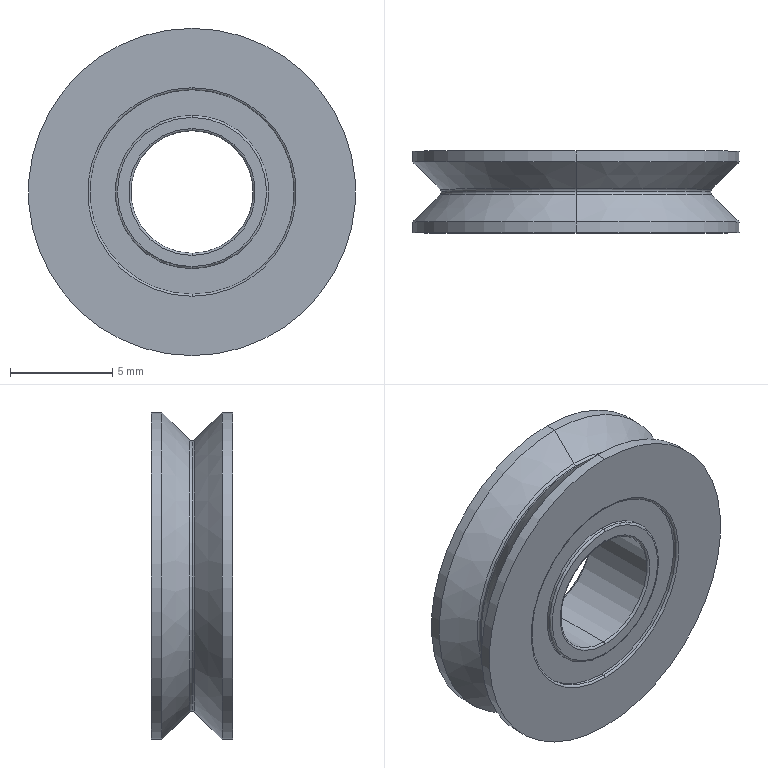Part | NX | features BREP 1 | 1 solid | 40 faces | box 16 x 4 x 16 mm | volume 572.042 mm3 | torus 16 | cylinder 14 | plane 6 | cone 4 | commonest cylinder face diameters 7.5 x4 10 x4 16 x4 6 x2
STEP:
#1=CARTESIAN_POINT('',(0.,2.,-6.613));
#2=VERTEX_POINT('',#1);
#3=CARTESIAN_POINT('',(0.,2.,6.613));
#4=VERTEX_POINT('',#3);
#5=CARTESIAN_POINT('',(0.,2.,0.));
#6=DIRECTION('',(0.,-1.,0.));
#7=DIRECTION('',(0.,0.,-1.));
#8=AXIS2_PLACEMENT_3D('',#5,#6,#7);
#9=CIRCLE('',#8,6.613);
#10=EDGE_CURVE('',#2,#4,#9,.T.);
#11=ORIENTED_EDGE('',*,*,#10,.F.);
#12=CARTESIAN_POINT('',(0.,2.141,-6.671));
#13=VERTEX_POINT('',#12);
#14=CARTESIAN_POINT('',(0.,2.,-6.813));
#15=DIRECTION('',(-1.,0.,0.));
#16=DIRECTION('',(0.,0.,1.));
#17=AXIS2_PLACEMENT_3D('',#14,#15,#16);
#18=CIRCLE('',#17,0.2);
#19=EDGE_CURVE('',#2,#13,#18,.T.);
#20=ORIENTED_EDGE('',*,*,#19,.T.);
#21=CARTESIAN_POINT('',(0.,2.141,6.671));
#22=VERTEX_POINT('',#21);
#23=CARTESIAN_POINT('',(0.,2.141,0.));
#24=DIRECTION('',(0.,1.,0.));
#25=DIRECTION('',(0.,0.,1.));
#26=AXIS2_PLACEMENT_3D('',#23,#24,#25);
#27=CIRCLE('',#26,6.671);
#28=EDGE_CURVE('',#22,#13,#27,.T.);
#29=ORIENTED_EDGE('',*,*,#28,.F.);
#30=CARTESIAN_POINT('',(0.,2.,6.813));
#31=DIRECTION('',(1.,0.,0.));
#32=DIRECTION('',(0.,0.,-1.));
#33=AXIS2_PLACEMENT_3D('',#30,#31,#32);
#34=CIRCLE('',#33,0.2);
#35=EDGE_CURVE('',#4,#22,#34,.T.);
#36=ORIENTED_EDGE('',*,*,#35,.F.);
#37=EDGE_LOOP('',(#11,#20,#29,#36));
#38=FACE_BOUND('',#37,.T.);
#39=CARTESIAN_POINT('',(0.,2.,0.));
#40=DIRECTION('',(0.,-1.,0.));
#41=DIRECTION('',(0.,0.,-1.));
#42=AXIS2_PLACEMENT_3D('',#39,#40,#41);
#43=TOROIDAL_SURFACE('',#42,6.813,0.2);
#44=ADVANCED_FACE('',(#38),#43,.F.);
#45=CARTESIAN_POINT('',(0.,3.9,-3.));
#46=VERTEX_POINT('',#45);
#47=CARTESIAN_POINT('',(0.,4.,-3.1));
#48=VERTEX_POINT('',#47);
#49=CARTESIAN_POINT('',(0.,3.9,-3.1));
#50=DIRECTION('',(1.,0.,0.));
#51=DIRECTION('',(0.,0.,-1.));
#52=AXIS2_PLACEMENT_3D('',#49,#50,#51);
#53=CIRCLE('',#52,0.1);
#54=EDGE_CURVE('',#46,#48,#53,.F.);
#55=ORIENTED_EDGE('',*,*,#54,.T.);
#56=CARTESIAN_POINT('',(0.,4.,3.1));
#57=VERTEX_POINT('',#56);
#58=CARTESIAN_POINT('',(0.,4.,0.));
#59=DIRECTION('',(0.,-1.,0.));
#60=DIRECTION('',(0.,0.,1.));
#61=AXIS2_PLACEMENT_3D('',#58,#59,#60);
#62=CIRCLE('',#61,3.1);
#63=EDGE_CURVE('',#57,#48,#62,.T.);
#64=ORIENTED_EDGE('',*,*,#63,.F.);
#65=CARTESIAN_POINT('',(0.,3.9,3.));
#66=VERTEX_POINT('',#65);
#67=CARTESIAN_POINT('',(0.,3.9,3.1));
#68=DIRECTION('',(-1.,0.,0.));
#69=DIRECTION('',(0.,0.,1.));
#70=AXIS2_PLACEMENT_3D('',#67,#68,#69);
#71=CIRCLE('',#70,0.1);
#72=EDGE_CURVE('',#66,#57,#71,.F.);
#73=ORIENTED_EDGE('',*,*,#72,.F.);
#74=CARTESIAN_POINT('',(0.,3.9,0.));
#75=DIRECTION('',(0.,1.,0.));
#76=DIRECTION('',(0.,0.,1.));
#77=AXIS2_PLACEMENT_3D('',#74,#75,#76);
#78=CIRCLE('',#77,3.);
#79=EDGE_CURVE('',#46,#66,#78,.T.);
#80=ORIENTED_EDGE('',*,*,#79,.F.);
#81=EDGE_LOOP('',(#55,#64,#73,#80));
#82=FACE_BOUND('',#81,.T.);
#83=CARTESIAN_POINT('',(0.,3.9,0.));
#84=DIRECTION('',(0.,1.,0.));
#85=DIRECTION('',(0.,0.,1.));
#86=AXIS2_PLACEMENT_3D('',#83,#84,#85);
#87=TOROIDAL_SURFACE('',#86,3.1,0.1);
#88=ADVANCED_FACE('',(#82),#87,.T.);
#89=CARTESIAN_POINT('',(0.,0.,3.1));
#90=VERTEX_POINT('',#89);
#91=CARTESIAN_POINT('',(0.,0.1,3.));
#92=VERTEX_POINT('',#91);
#93=CARTESIAN_POINT('',(0.,0.1,3.1));
#94=DIRECTION('',(1.,0.,0.));
#95=DIRECTION('',(0.,0.,-1.));
#96=AXIS2_PLACEMENT_3D('',#93,#94,#95);
#97=CIRCLE('',#96,0.1);
#98=EDGE_CURVE('',#90,#92,#97,.T.);
#99=ORIENTED_EDGE('',*,*,#98,.F.);
#100=CARTESIAN_POINT('',(0.,0.,-3.1));
#101=VERTEX_POINT('',#100);
#102=CARTESIAN_POINT('',(0.,0.,0.));
#103=DIRECTION('',(0.,1.,0.));
#104=DIRECTION('',(0.,0.,-1.));
#105=AXIS2_PLACEMENT_3D('',#102,#103,#104);
#106=CIRCLE('',#105,3.1);
#107=EDGE_CURVE('',#101,#90,#106,.T.);
#108=ORIENTED_EDGE('',*,*,#107,.F.);
#109=CARTESIAN_POINT('',(0.,0.1,-3.));
#110=VERTEX_POINT('',#109);
#111=CARTESIAN_POINT('',(0.,0.1,-3.1));
#112=DIRECTION('',(-1.,0.,0.));
#113=DIRECTION('',(0.,0.,1.));
#114=AXIS2_PLACEMENT_3D('',#111,#112,#113);
#115=CIRCLE('',#114,0.1);
#116=EDGE_CURVE('',#101,#110,#115,.T.);
#117=ORIENTED_EDGE('',*,*,#116,.T.);
#118=CARTESIAN_POINT('',(0.,0.1,0.));
#119=DIRECTION('',(0.,-1.,0.));
#120=DIRECTION('',(0.,0.,-1.));
#121=AXIS2_PLACEMENT_3D('',#118,#119,#120);
#122=CIRCLE('',#121,3.);
#123=EDGE_CURVE('',#92,#110,#122,.T.);
#124=ORIENTED_EDGE('',*,*,#123,.F.);
#125=EDGE_LOOP('',(#99,#108,#117,#124));
#126=FACE_BOUND('',#125,.T.);
#127=CARTESIAN_POINT('',(0.,0.1,0.));
#128=DIRECTION('',(0.,-1.,0.));
#129=DIRECTION('',(0.,0.,-1.));
#130=AXIS2_PLACEMENT_3D('',#127,#128,#129);
#131=TOROIDAL_SURFACE('',#130,3.1,0.1);
#132=ADVANCED_FACE('',(#126),#131,.T.);
#133=CARTESIAN_POINT('',(0.,4.,-3.65));
#134=VERTEX_POINT('',#133);
#135=CARTESIAN_POINT('',(0.,3.9,-3.75));
#136=VERTEX_POINT('',#135);
#137=CARTESIAN_POINT('',(0.,3.9,-3.65));
#138=DIRECTION('',(1.,0.,0.));
#139=DIRECTION('',(0.,0.,-1.));
#140=AXIS2_PLACEMENT_3D('',#137,#138,#139);
#141=CIRCLE('',#140,0.1);
#142=EDGE_CURVE('',#134,#136,#141,.F.);
#143=ORIENTED_EDGE('',*,*,#142,.T.);
#144=CARTESIAN_POINT('',(0.,3.9,3.75));
#145=VERTEX_POINT('',#144);
#146=CARTESIAN_POINT('',(0.,3.9,0.));
#147=DIRECTION('',(0.,-1.,0.));
#148=DIRECTION('',(0.,0.,1.));
#149=AXIS2_PLACEMENT_3D('',#146,#147,#148);
#150=CIRCLE('',#149,3.75);
#151=EDGE_CURVE('',#145,#136,#150,.T.);
#152=ORIENTED_EDGE('',*,*,#151,.F.);
#153=CARTESIAN_POINT('',(0.,4.,3.65));
#154=VERTEX_POINT('',#153);
#155=CARTESIAN_POINT('',(0.,3.9,3.65));
#156=DIRECTION('',(-1.,0.,0.));
#157=DIRECTION('',(0.,0.,1.));
#158=AXIS2_PLACEMENT_3D('',#155,#156,#157);
#159=CIRCLE('',#158,0.1);
#160=EDGE_CURVE('',#154,#145,#159,.F.);
#161=ORIENTED_EDGE('',*,*,#160,.F.);
#162=CARTESIAN_POINT('',(0.,4.,0.));
#163=DIRECTION('',(0.,1.,0.));
#164=DIRECTION('',(0.,0.,1.));
#165=AXIS2_PLACEMENT_3D('',#162,#163,#164);
#166=CIRCLE('',#165,3.65);
#167=EDGE_CURVE('',#134,#154,#166,.T.);
#168=ORIENTED_EDGE('',*,*,#167,.F.);
#169=EDGE_LOOP('',(#143,#152,#161,#168));
#170=FACE_BOUND('',#169,.T.);
#171=CARTESIAN_POINT('',(0.,3.9,0.));
#172=DIRECTION('',(0.,1.,0.));
#173=DIRECTION('',(0.,0.,1.));
#174=AXIS2_PLACEMENT_3D('',#171,#172,#173);
#175=TOROIDAL_SURFACE('',#174,3.65,0.1);
#176=ADVANCED_FACE('',(#170),#175,.T.);
#177=CARTESIAN_POINT('',(0.,3.9,-5.));
#178=VERTEX_POINT('',#177);
#179=CARTESIAN_POINT('',(0.,4.,-5.1));
#180=VERTEX_POINT('',#179);
#181=CARTESIAN_POINT('',(0.,3.9,-5.1));
#182=DIRECTION('',(1.,0.,0.));
#183=DIRECTION('',(0.,0.,-1.));
#184=AXIS2_PLACEMENT_3D('',#181,#182,#183);
#185=CIRCLE('',#184,0.1);
#186=EDGE_CURVE('',#178,#180,#185,.F.);
#187=ORIENTED_EDGE('',*,*,#186,.T.);
#188=CARTESIAN_POINT('',(0.,4.,5.1));
#189=VERTEX_POINT('',#188);
#190=CARTESIAN_POINT('',(0.,4.,0.));
#191=DIRECTION('',(0.,-1.,0.));
#192=DIRECTION('',(0.,0.,1.));
#193=AXIS2_PLACEMENT_3D('',#190,#191,#192);
#194=CIRCLE('',#193,5.1);
#195=EDGE_CURVE('',#189,#180,#194,.T.);
#196=ORIENTED_EDGE('',*,*,#195,.F.);
#197=CARTESIAN_POINT('',(0.,3.9,5.));
#198=VERTEX_POINT('',#197);
#199=CARTESIAN_POINT('',(0.,3.9,5.1));
#200=DIRECTION('',(-1.,0.,0.));
#201=DIRECTION('',(0.,0.,1.));
#202=AXIS2_PLACEMENT_3D('',#199,#200,#201);
#203=CIRCLE('',#202,0.1);
#204=EDGE_CURVE('',#198,#189,#203,.F.);
#205=ORIENTED_EDGE('',*,*,#204,.F.);
#206=CARTESIAN_POINT('',(0.,3.9,0.));
#207=DIRECTION('',(0.,1.,0.));
#208=DIRECTION('',(0.,0.,1.));
#209=AXIS2_PLACEMENT_3D('',#206,#207,#208);
#210=CIRCLE('',#209,5.);
#211=EDGE_CURVE('',#178,#198,#210,.T.);
#212=ORIENTED_EDGE('',*,*,#211,.F.);
#213=EDGE_LOOP('',(#187,#196,#205,#212));
#214=FACE_BOUND('',#213,.T.);
#215=CARTESIAN_POINT('',(0.,3.9,0.));
#216=DIRECTION('',(0.,1.,0.));
#217=DIRECTION('',(0.,0.,1.));
#218=AXIS2_PLACEMENT_3D('',#215,#216,#217);
#219=TOROIDAL_SURFACE('',#218,5.1,0.1);
#220=ADVANCED_FACE('',(#214),#219,.T.);
#221=CARTESIAN_POINT('',(0.,0.1,3.75));
#222=VERTEX_POINT('',#221);
#223=CARTESIAN_POINT('',(0.,0.,3.65));
#224=VERTEX_POINT('',#223);
#225=CARTESIAN_POINT('',(0.,0.1,3.65));
#226=DIRECTION('',(1.,0.,0.));
#227=DIRECTION('',(0.,0.,-1.));
#228=AXIS2_PLACEMENT_3D('',#225,#226,#227);
#229=CIRCLE('',#228,0.1);
#230=EDGE_CURVE('',#222,#224,#229,.T.);
#231=ORIENTED_EDGE('',*,*,#230,.F.);
#232=CARTESIAN_POINT('',(0.,0.1,-3.75));
#233=VERTEX_POINT('',#232);
#234=CARTESIAN_POINT('',(0.,0.1,0.));
#235=DIRECTION('',(0.,1.,0.));
#236=DIRECTION('',(0.,0.,-1.));
#237=AXIS2_PLACEMENT_3D('',#234,#235,#236);
#238=CIRCLE('',#237,3.75);
#239=EDGE_CURVE('',#233,#222,#238,.T.);
#240=ORIENTED_EDGE('',*,*,#239,.F.);
#241=CARTESIAN_POINT('',(0.,0.,-3.65));
#242=VERTEX_POINT('',#241);
#243=CARTESIAN_POINT('',(0.,0.1,-3.65));
#244=DIRECTION('',(-1.,0.,0.));
#245=DIRECTION('',(0.,0.,1.));
#246=AXIS2_PLACEMENT_3D('',#243,#244,#245);
#247=CIRCLE('',#246,0.1);
#248=EDGE_CURVE('',#233,#242,#247,.T.);
#249=ORIENTED_EDGE('',*,*,#248,.T.);
#250=CARTESIAN_POINT('',(0.,0.,0.));
#251=DIRECTION('',(0.,-1.,0.));
#252=DIRECTION('',(0.,0.,-1.));
#253=AXIS2_PLACEMENT_3D('',#250,#251,#252);
#254=CIRCLE('',#253,3.65);
#255=EDGE_CURVE('',#224,#242,#254,.T.);
#256=ORIENTED_EDGE('',*,*,#255,.F.);
#257=EDGE_LOOP('',(#231,#240,#249,#256));
#258=FACE_BOUND('',#257,.T.);
#259=CARTESIAN_POINT('',(0.,0.1,0.));
#260=DIRECTION('',(0.,-1.,0.));
#261=DIRECTION('',(0.,0.,-1.));
#262=AXIS2_PLACEMENT_3D('',#259,#260,#261);
#263=TOROIDAL_SURFACE('',#262,3.65,0.1);
#264=ADVANCED_FACE('',(#258),#263,.T.);
#265=CARTESIAN_POINT('',(0.,0.,5.1));
#266=VERTEX_POINT('',#265);
#267=CARTESIAN_POINT('',(0.,0.1,5.));
#268=VERTEX_POINT('',#267);
#269=CARTESIAN_POINT('',(0.,0.1,5.1));
#270=DIRECTION('',(1.,0.,0.));
#271=DIRECTION('',(0.,0.,-1.));
#272=AXIS2_PLACEMENT_3D('',#269,#270,#271);
#273=CIRCLE('',#272,0.1);
#274=EDGE_CURVE('',#266,#268,#273,.T.);
#275=ORIENTED_EDGE('',*,*,#274,.F.);
#276=CARTESIAN_POINT('',(0.,0.,-5.1));
#277=VERTEX_POINT('',#276);
#278=CARTESIAN_POINT('',(0.,0.,0.));
#279=DIRECTION('',(0.,1.,0.));
#280=DIRECTION('',(0.,0.,-1.));
#281=AXIS2_PLACEMENT_3D('',#278,#279,#280);
#282=CIRCLE('',#281,5.1);
#283=EDGE_CURVE('',#277,#266,#282,.T.);
#284=ORIENTED_EDGE('',*,*,#283,.F.);
#285=CARTESIAN_POINT('',(0.,0.1,-5.));
#286=VERTEX_POINT('',#285);
#287=CARTESIAN_POINT('',(0.,0.1,-5.1));
#288=DIRECTION('',(-1.,0.,0.));
#289=DIRECTION('',(0.,0.,1.));
#290=AXIS2_PLACEMENT_3D('',#287,#288,#289);
#291=CIRCLE('',#290,0.1);
#292=EDGE_CURVE('',#277,#286,#291,.T.);
#293=ORIENTED_EDGE('',*,*,#292,.T.);
#294=CARTESIAN_POINT('',(0.,0.1,0.));
#295=DIRECTION('',(0.,-1.,0.));
#296=DIRECTION('',(0.,0.,-1.));
#297=AXIS2_PLACEMENT_3D('',#294,#295,#296);
#298=CIRCLE('',#297,5.);
#299=EDGE_CURVE('',#268,#286,#298,.T.);
#300=ORIENTED_EDGE('',*,*,#299,.F.);
#301=EDGE_LOOP('',(#275,#284,#293,#300));
#302=FACE_BOUND('',#301,.T.);
#303=CARTESIAN_POINT('',(0.,0.1,0.));
#304=DIRECTION('',(0.,-1.,0.));
#305=DIRECTION('',(0.,0.,-1.));
#306=AXIS2_PLACEMENT_3D('',#303,#304,#305);
#307=TOROIDAL_SURFACE('',#306,5.1,0.1);
#308=ADVANCED_FACE('',(#302),#307,.T.);
#309=CARTESIAN_POINT('',(0.,3.75,-3.75));
#310=VERTEX_POINT('',#309);
#311=CARTESIAN_POINT('',(0.,3.75,-3.75));
#312=DIRECTION('',(0.,1.,0.));
#313=VECTOR('',#312,1000.);
#314=LINE('',#311,#313);
#315=EDGE_CURVE('',#136,#310,#314,.F.);
#316=ORIENTED_EDGE('',*,*,#315,.T.);
#317=CARTESIAN_POINT('',(0.,3.75,3.75));
#318=VERTEX_POINT('',#317);
#319=CARTESIAN_POINT('',(0.,3.75,0.));
#320=DIRECTION('',(0.,1.,0.));
#321=DIRECTION('',(0.,0.,1.));
#322=AXIS2_PLACEMENT_3D('',#319,#320,#321);
#323=CIRCLE('',#322,3.75);
#324=EDGE_CURVE('',#310,#318,#323,.T.);
#325=ORIENTED_EDGE('',*,*,#324,.T.);
#326=CARTESIAN_POINT('',(0.,3.75,3.75));
#327=DIRECTION('',(0.,1.,0.));
#328=VECTOR('',#327,1000.);
#329=LINE('',#326,#328);
#330=EDGE_CURVE('',#145,#318,#329,.F.);
#331=ORIENTED_EDGE('',*,*,#330,.F.);
#332=ORIENTED_EDGE('',*,*,#151,.T.);
#333=EDGE_LOOP('',(#316,#325,#331,#332));
#334=FACE_BOUND('',#333,.T.);
#335=CARTESIAN_POINT('',(0.,3.75,0.));
#336=DIRECTION('',(0.,1.,0.));
#337=DIRECTION('',(0.,0.,1.));
#338=AXIS2_PLACEMENT_3D('',#335,#336,#337);
#339=CYLINDRICAL_SURFACE('',#338,3.75);
#340=ADVANCED_FACE('',(#334),#339,.T.);
#341=CARTESIAN_POINT('',(0.,3.75,5.));
#342=VERTEX_POINT('',#341);
#343=CARTESIAN_POINT('',(0.,3.75,-5.));
#344=VERTEX_POINT('',#343);
#345=CARTESIAN_POINT('',(0.,3.75,0.));
#346=DIRECTION('',(0.,1.,0.));
#347=DIRECTION('',(0.,0.,1.));
#348=AXIS2_PLACEMENT_3D('',#345,#346,#347);
#349=CIRCLE('',#348,5.);
#350=EDGE_CURVE('',#342,#344,#349,.T.);
#351=ORIENTED_EDGE('',*,*,#350,.T.);
#352=CARTESIAN_POINT('',(0.,3.75,0.));
#353=DIRECTION('',(0.,1.,0.));
#354=DIRECTION('',(0.,0.,1.));
#355=AXIS2_PLACEMENT_3D('',#352,#353,#354);
#356=CIRCLE('',#355,5.);
#357=EDGE_CURVE('',#344,#342,#356,.T.);
#358=ORIENTED_EDGE('',*,*,#357,.T.);
#359=EDGE_LOOP('',(#351,#358));
#360=FACE_BOUND('',#359,.T.);
#361=CARTESIAN_POINT('',(0.,3.75,0.));
#362=DIRECTION('',(0.,1.,0.));
#363=DIRECTION('',(0.,0.,1.));
#364=AXIS2_PLACEMENT_3D('',#361,#362,#363);
#365=CIRCLE('',#364,3.75);
#366=EDGE_CURVE('',#318,#310,#365,.T.);
#367=ORIENTED_EDGE('',*,*,#366,.F.);
#368=ORIENTED_EDGE('',*,*,#324,.F.);
#369=EDGE_LOOP('',(#367,#368));
#370=FACE_BOUND('',#369,.T.);
#371=CARTESIAN_POINT('',(0.,3.75,0.));
#372=DIRECTION('',(0.,1.,0.));
#373=DIRECTION('',(0.,0.,1.));
#374=AXIS2_PLACEMENT_3D('',#371,#372,#373);
#375=PLANE('',#374);
#376=ADVANCED_FACE('',(#360,#370),#375,.T.);
#377=CARTESIAN_POINT('',(0.,3.75,-5.));
#378=DIRECTION('',(0.,1.,0.));
#379=VECTOR('',#378,1000.);
#380=LINE('',#377,#379);
#381=EDGE_CURVE('',#178,#344,#380,.F.);
#382=ORIENTED_EDGE('',*,*,#381,.T.);
#383=ORIENTED_EDGE('',*,*,#350,.F.);
#384=CARTESIAN_POINT('',(0.,3.75,5.));
#385=DIRECTION('',(0.,1.,0.));
#386=VECTOR('',#385,1000.);
#387=LINE('',#384,#386);
#388=EDGE_CURVE('',#198,#342,#387,.F.);
#389=ORIENTED_EDGE('',*,*,#388,.F.);
#390=CARTESIAN_POINT('',(0.,3.9,0.));
#391=DIRECTION('',(0.,1.,0.));
#392=DIRECTION('',(0.,0.,1.));
#393=AXIS2_PLACEMENT_3D('',#390,#391,#392);
#394=CIRCLE('',#393,5.);
#395=EDGE_CURVE('',#198,#178,#394,.T.);
#396=ORIENTED_EDGE('',*,*,#395,.T.);
#397=EDGE_LOOP('',(#382,#383,#389,#396));
#398=FACE_BOUND('',#397,.T.);
#399=CARTESIAN_POINT('',(0.,3.75,0.));
#400=DIRECTION('',(0.,1.,0.));
#401=DIRECTION('',(0.,0.,1.));
#402=AXIS2_PLACEMENT_3D('',#399,#400,#401);
#403=CYLINDRICAL_SURFACE('',#402,5.);
#404=ADVANCED_FACE('',(#398),#403,.F.);
#405=CARTESIAN_POINT('',(0.,0.25,3.75));
#406=VERTEX_POINT('',#405);
#407=CARTESIAN_POINT('',(0.,0.25,3.75));
#408=DIRECTION('',(0.,-1.,0.));
#409=VECTOR('',#408,1000.);
#410=LINE('',#407,#409);
#411=EDGE_CURVE('',#406,#222,#410,.T.);
#412=ORIENTED_EDGE('',*,*,#411,.F.);
#413=CARTESIAN_POINT('',(0.,0.25,-3.75));
#414=VERTEX_POINT('',#413);
#415=CARTESIAN_POINT('',(0.,0.25,0.));
#416=DIRECTION('',(0.,-1.,0.));
#417=DIRECTION('',(0.,0.,-1.));
#418=AXIS2_PLACEMENT_3D('',#415,#416,#417);
#419=CIRCLE('',#418,3.75);
#420=EDGE_CURVE('',#406,#414,#419,.T.);
#421=ORIENTED_EDGE('',*,*,#420,.T.);
#422=CARTESIAN_POINT('',(0.,0.25,-3.75));
#423=DIRECTION('',(0.,-1.,0.));
#424=VECTOR('',#423,1000.);
#425=LINE('',#422,#424);
#426=EDGE_CURVE('',#414,#233,#425,.T.);
#427=ORIENTED_EDGE('',*,*,#426,.T.);
#428=ORIENTED_EDGE('',*,*,#239,.T.);
#429=EDGE_LOOP('',(#412,#421,#427,#428));
#430=FACE_BOUND('',#429,.T.);
#431=CARTESIAN_POINT('',(0.,0.25,0.));
#432=DIRECTION('',(0.,-1.,0.));
#433=DIRECTION('',(0.,0.,-1.));
#434=AXIS2_PLACEMENT_3D('',#431,#432,#433);
#435=CYLINDRICAL_SURFACE('',#434,3.75);
#436=ADVANCED_FACE('',(#430),#435,.T.);
#437=CARTESIAN_POINT('',(0.,0.25,-5.));
#438=VERTEX_POINT('',#437);
#439=CARTESIAN_POINT('',(0.,0.25,5.));
#440=VERTEX_POINT('',#439);
#441=CARTESIAN_POINT('',(0.,0.25,0.));
#442=DIRECTION('',(0.,-1.,0.));
#443=DIRECTION('',(0.,0.,-1.));
#444=AXIS2_PLACEMENT_3D('',#441,#442,#443);
#445=CIRCLE('',#444,5.);
#446=EDGE_CURVE('',#438,#440,#445,.T.);
#447=ORIENTED_EDGE('',*,*,#446,.T.);
#448=CARTESIAN_POINT('',(0.,0.25,0.));
#449=DIRECTION('',(0.,-1.,0.));
#450=DIRECTION('',(0.,0.,-1.));
#451=AXIS2_PLACEMENT_3D('',#448,#449,#450);
#452=CIRCLE('',#451,5.);
#453=EDGE_CURVE('',#440,#438,#452,.T.);
#454=ORIENTED_EDGE('',*,*,#453,.T.);
#455=EDGE_LOOP('',(#447,#454));
#456=FACE_BOUND('',#455,.T.);
#457=CARTESIAN_POINT('',(0.,0.25,0.));
#458=DIRECTION('',(0.,-1.,0.));
#459=DIRECTION('',(0.,0.,-1.));
#460=AXIS2_PLACEMENT_3D('',#457,#458,#459);
#461=CIRCLE('',#460,3.75);
#462=EDGE_CURVE('',#414,#406,#461,.T.);
#463=ORIENTED_EDGE('',*,*,#462,.F.);
#464=ORIENTED_EDGE('',*,*,#420,.F.);
#465=EDGE_LOOP('',(#463,#464));
#466=FACE_BOUND('',#465,.T.);
#467=CARTESIAN_POINT('',(0.,0.25,0.));
#468=DIRECTION('',(0.,-1.,0.));
#469=DIRECTION('',(0.,0.,-1.));
#470=AXIS2_PLACEMENT_3D('',#467,#468,#469);
#471=PLANE('',#470);
#472=ADVANCED_FACE('',(#456,#466),#471,.T.);
#473=CARTESIAN_POINT('',(0.,0.25,5.));
#474=DIRECTION('',(0.,-1.,0.));
#475=VECTOR('',#474,1000.);
#476=LINE('',#473,#475);
#477=EDGE_CURVE('',#440,#268,#476,.T.);
#478=ORIENTED_EDGE('',*,*,#477,.F.);
#479=ORIENTED_EDGE('',*,*,#446,.F.);
#480=CARTESIAN_POINT('',(0.,0.25,-5.));
#481=DIRECTION('',(0.,-1.,0.));
#482=VECTOR('',#481,1000.);
#483=LINE('',#480,#482);
#484=EDGE_CURVE('',#438,#286,#483,.T.);
#485=ORIENTED_EDGE('',*,*,#484,.T.);
#486=CARTESIAN_POINT('',(0.,0.1,0.));
#487=DIRECTION('',(0.,-1.,0.));
#488=DIRECTION('',(0.,0.,-1.));
#489=AXIS2_PLACEMENT_3D('',#486,#487,#488);
#490=CIRCLE('',#489,5.);
#491=EDGE_CURVE('',#286,#268,#490,.T.);
#492=ORIENTED_EDGE('',*,*,#491,.T.);
#493=EDGE_LOOP('',(#478,#479,#485,#492));
#494=FACE_BOUND('',#493,.T.);
#495=CARTESIAN_POINT('',(0.,0.25,0.));
#496=DIRECTION('',(0.,-1.,0.));
#497=DIRECTION('',(0.,0.,-1.));
#498=AXIS2_PLACEMENT_3D('',#495,#496,#497);
#499=CYLINDRICAL_SURFACE('',#498,5.);
#500=ADVANCED_FACE('',(#494),#499,.F.);
#501=CARTESIAN_POINT('',(0.,0.53,8.));
#502=VERTEX_POINT('',#501);
#503=CARTESIAN_POINT('',(0.,0.,8.));
#504=VERTEX_POINT('',#503);
#505=CARTESIAN_POINT('',(0.,0.,8.));
#506=DIRECTION('',(0.,-1.,0.));
#507=VECTOR('',#506,1000.);
#508=LINE('',#505,#507);
#509=EDGE_CURVE('',#502,#504,#508,.T.);
#510=ORIENTED_EDGE('',*,*,#509,.F.);
#511=CARTESIAN_POINT('',(0.,0.53,-8.));
#512=VERTEX_POINT('',#511);
#513=CARTESIAN_POINT('',(0.,0.53,0.));
#514=DIRECTION('',(0.,-1.,0.));
#515=DIRECTION('',(0.,0.,-1.));
#516=AXIS2_PLACEMENT_3D('',#513,#514,#515);
#517=CIRCLE('',#516,8.);
#518=EDGE_CURVE('',#502,#512,#517,.T.);
#519=ORIENTED_EDGE('',*,*,#518,.T.);
#520=CARTESIAN_POINT('',(0.,0.,-8.));
#521=VERTEX_POINT('',#520);
#522=CARTESIAN_POINT('',(0.,0.,-8.));
#523=DIRECTION('',(0.,-1.,0.));
#524=VECTOR('',#523,1000.);
#525=LINE('',#522,#524);
#526=EDGE_CURVE('',#512,#521,#525,.T.);
#527=ORIENTED_EDGE('',*,*,#526,.T.);
#528=CARTESIAN_POINT('',(0.,0.,0.));
#529=DIRECTION('',(0.,-1.,0.));
#530=DIRECTION('',(0.,0.,-1.));
#531=AXIS2_PLACEMENT_3D('',#528,#529,#530);
#532=CIRCLE('',#531,8.);
#533=EDGE_CURVE('',#504,#521,#532,.T.);
#534=ORIENTED_EDGE('',*,*,#533,.F.);
#535=EDGE_LOOP('',(#510,#519,#527,#534));
#536=FACE_BOUND('',#535,.T.);
#537=CARTESIAN_POINT('',(0.,0.,0.));
#538=DIRECTION('',(0.,-1.,0.));
#539=DIRECTION('',(0.,0.,-1.));
#540=AXIS2_PLACEMENT_3D('',#537,#538,#539);
#541=CYLINDRICAL_SURFACE('',#540,8.);
#542=ADVANCED_FACE('',(#536),#541,.T.);
#543=CARTESIAN_POINT('',(0.,1.859,6.671));
#544=VERTEX_POINT('',#543);
#545=CARTESIAN_POINT('',(0.,0.53,8.));
#546=DIRECTION('',(0.,-0.7071,0.7071));
#547=VECTOR('',#546,1000.);
#548=LINE('',#545,#547);
#549=EDGE_CURVE('',#544,#502,#548,.T.);
#550=ORIENTED_EDGE('',*,*,#549,.F.);
#551=CARTESIAN_POINT('',(0.,1.859,-6.671));
#552=VERTEX_POINT('',#551);
#553=CARTESIAN_POINT('',(0.,1.859,0.));
#554=DIRECTION('',(0.,-1.,0.));
#555=DIRECTION('',(0.,0.,-1.));
#556=AXIS2_PLACEMENT_3D('',#553,#554,#555);
#557=CIRCLE('',#556,6.671);
#558=EDGE_CURVE('',#544,#552,#557,.T.);
#559=ORIENTED_EDGE('',*,*,#558,.T.);
#560=CARTESIAN_POINT('',(0.,0.53,-8.));
#561=DIRECTION('',(0.,-0.7071,-0.7071));
#562=VECTOR('',#561,1000.);
#563=LINE('',#560,#562);
#564=EDGE_CURVE('',#552,#512,#563,.T.);
#565=ORIENTED_EDGE('',*,*,#564,.T.);
#566=ORIENTED_EDGE('',*,*,#518,.F.);
#567=EDGE_LOOP('',(#550,#559,#565,#566));
#568=FACE_BOUND('',#567,.T.);
#569=CARTESIAN_POINT('',(0.,0.53,0.));
#570=DIRECTION('',(0.,-1.,0.));
#571=DIRECTION('',(0.,0.,-1.));
#572=AXIS2_PLACEMENT_3D('',#569,#570,#571);
#573=CONICAL_SURFACE('',#572,8.,0.7854);
#574=ADVANCED_FACE('',(#568),#573,.T.);
#575=CARTESIAN_POINT('',(0.,3.47,-8.));
#576=VERTEX_POINT('',#575);
#577=CARTESIAN_POINT('',(0.,2.,-6.53));
#578=DIRECTION('',(0.,0.7071,-0.7071));
#579=VECTOR('',#578,1000.);
#580=LINE('',#577,#579);
#581=EDGE_CURVE('',#576,#13,#580,.F.);
#582=ORIENTED_EDGE('',*,*,#581,.T.);
#583=CARTESIAN_POINT('',(0.,2.141,0.));
#584=DIRECTION('',(0.,1.,0.));
#585=DIRECTION('',(0.,0.,1.));
#586=AXIS2_PLACEMENT_3D('',#583,#584,#585);
#587=CIRCLE('',#586,6.671);
#588=EDGE_CURVE('',#13,#22,#587,.T.);
#589=ORIENTED_EDGE('',*,*,#588,.T.);
#590=CARTESIAN_POINT('',(0.,3.47,8.));
#591=VERTEX_POINT('',#590);
#592=CARTESIAN_POINT('',(0.,2.,6.53));
#593=DIRECTION('',(0.,0.7071,0.7071));
#594=VECTOR('',#593,1000.);
#595=LINE('',#592,#594);
#596=EDGE_CURVE('',#591,#22,#595,.F.);
#597=ORIENTED_EDGE('',*,*,#596,.F.);
#598=CARTESIAN_POINT('',(0.,3.47,0.));
#599=DIRECTION('',(0.,-1.,0.));
#600=DIRECTION('',(0.,0.,-1.));
#601=AXIS2_PLACEMENT_3D('',#598,#599,#600);
#602=CIRCLE('',#601,8.);
#603=EDGE_CURVE('',#591,#576,#602,.T.);
#604=ORIENTED_EDGE('',*,*,#603,.T.);
#605=EDGE_LOOP('',(#582,#589,#597,#604));
#606=FACE_BOUND('',#605,.T.);
#607=CARTESIAN_POINT('',(0.,2.,0.));
#608=DIRECTION('',(0.,1.,0.));
#609=DIRECTION('',(0.,0.,1.));
#610=AXIS2_PLACEMENT_3D('',#607,#608,#609);
#611=CONICAL_SURFACE('',#610,6.53,0.7854);
#612=ADVANCED_FACE('',(#606),#611,.T.);
#613=CARTESIAN_POINT('',(0.,4.,8.));
#614=VERTEX_POINT('',#613);
#615=CARTESIAN_POINT('',(0.,0.,8.));
#616=DIRECTION('',(0.,-1.,0.));
#617=VECTOR('',#616,1000.);
#618=LINE('',#615,#617);
#619=EDGE_CURVE('',#614,#591,#618,.T.);
#620=ORIENTED_EDGE('',*,*,#619,.F.);
#621=CARTESIAN_POINT('',(0.,4.,-8.));
#622=VERTEX_POINT('',#621);
#623=CARTESIAN_POINT('',(0.,4.,0.));
#624=DIRECTION('',(0.,-1.,0.));
#625=DIRECTION('',(0.,0.,-1.));
#626=AXIS2_PLACEMENT_3D('',#623,#624,#625);
#627=CIRCLE('',#626,8.);
#628=EDGE_CURVE('',#614,#622,#627,.T.);
#629=ORIENTED_EDGE('',*,*,#628,.T.);
#630=CARTESIAN_POINT('',(0.,0.,-8.));
#631=DIRECTION('',(0.,-1.,0.));
#632=VECTOR('',#631,1000.);
#633=LINE('',#630,#632);
#634=EDGE_CURVE('',#622,#576,#633,.T.);
#635=ORIENTED_EDGE('',*,*,#634,.T.);
#636=ORIENTED_EDGE('',*,*,#603,.F.);
#637=EDGE_LOOP('',(#620,#629,#635,#636));
#638=FACE_BOUND('',#637,.T.);
#639=CARTESIAN_POINT('',(0.,0.,0.));
#640=DIRECTION('',(0.,-1.,0.));
#641=DIRECTION('',(0.,0.,-1.));
#642=AXIS2_PLACEMENT_3D('',#639,#640,#641);
#643=CYLINDRICAL_SURFACE('',#642,8.);
#644=ADVANCED_FACE('',(#638),#643,.T.);
#645=CARTESIAN_POINT('',(0.,4.,0.));
#646=DIRECTION('',(0.,-1.,0.));
#647=DIRECTION('',(0.,0.,-1.));
#648=AXIS2_PLACEMENT_3D('',#645,#646,#647);
#649=CIRCLE('',#648,8.);
#650=EDGE_CURVE('',#622,#614,#649,.T.);
#651=ORIENTED_EDGE('',*,*,#650,.F.);
#652=ORIENTED_EDGE('',*,*,#628,.F.);
#653=EDGE_LOOP('',(#651,#652));
#654=FACE_BOUND('',#653,.T.);
#655=ORIENTED_EDGE('',*,*,#195,.T.);
#656=CARTESIAN_POINT('',(0.,4.,0.));
#657=DIRECTION('',(0.,-1.,0.));
#658=DIRECTION('',(0.,0.,1.));
#659=AXIS2_PLACEMENT_3D('',#656,#657,#658);
#660=CIRCLE('',#659,5.1);
#661=EDGE_CURVE('',#180,#189,#660,.T.);
#662=ORIENTED_EDGE('',*,*,#661,.T.);
#663=EDGE_LOOP('',(#655,#662));
#664=FACE_BOUND('',#663,.T.);
#665=CARTESIAN_POINT('',(3.,4.,0.));
#666=DIRECTION('',(0.,1.,0.));
#667=DIRECTION('',(0.,0.,1.));
#668=AXIS2_PLACEMENT_3D('',#665,#666,#667);
#669=PLANE('',#668);
#670=ADVANCED_FACE('',(#654,#664),#669,.T.);
#671=CARTESIAN_POINT('',(0.,0.,3.));
#672=DIRECTION('',(0.,-1.,0.));
#673=VECTOR('',#672,1000.);
#674=LINE('',#671,#673);
#675=EDGE_CURVE('',#66,#92,#674,.T.);
#676=ORIENTED_EDGE('',*,*,#675,.F.);
#677=CARTESIAN_POINT('',(0.,3.9,0.));
#678=DIRECTION('',(0.,1.,0.));
#679=DIRECTION('',(0.,0.,1.));
#680=AXIS2_PLACEMENT_3D('',#677,#678,#679);
#681=CIRCLE('',#680,3.);
#682=EDGE_CURVE('',#66,#46,#681,.T.);
#683=ORIENTED_EDGE('',*,*,#682,.T.);
#684=CARTESIAN_POINT('',(0.,0.,-3.));
#685=DIRECTION('',(0.,-1.,0.));
#686=VECTOR('',#685,1000.);
#687=LINE('',#684,#686);
#688=EDGE_CURVE('',#46,#110,#687,.T.);
#689=ORIENTED_EDGE('',*,*,#688,.T.);
#690=CARTESIAN_POINT('',(0.,0.1,0.));
#691=DIRECTION('',(0.,-1.,0.));
#692=DIRECTION('',(0.,0.,-1.));
#693=AXIS2_PLACEMENT_3D('',#690,#691,#692);
#694=CIRCLE('',#693,3.);
#695=EDGE_CURVE('',#110,#92,#694,.T.);
#696=ORIENTED_EDGE('',*,*,#695,.T.);
#697=EDGE_LOOP('',(#676,#683,#689,#696));
#698=FACE_BOUND('',#697,.T.);
#699=CARTESIAN_POINT('',(0.,0.,0.));
#700=DIRECTION('',(0.,-1.,0.));
#701=DIRECTION('',(0.,0.,-1.));
#702=AXIS2_PLACEMENT_3D('',#699,#700,#701);
#703=CYLINDRICAL_SURFACE('',#702,3.);
#704=ADVANCED_FACE('',(#698),#703,.F.);
#705=CARTESIAN_POINT('',(0.,0.,0.));
#706=DIRECTION('',(0.,-1.,0.));
#707=DIRECTION('',(0.,0.,-1.));
#708=AXIS2_PLACEMENT_3D('',#705,#706,#707);
#709=CIRCLE('',#708,8.);
#710=EDGE_CURVE('',#521,#504,#709,.T.);
#711=ORIENTED_EDGE('',*,*,#710,.T.);
#712=ORIENTED_EDGE('',*,*,#533,.T.);
#713=EDGE_LOOP('',(#711,#712));
#714=FACE_BOUND('',#713,.T.);
#715=ORIENTED_EDGE('',*,*,#283,.T.);
#716=CARTESIAN_POINT('',(0.,0.,0.));
#717=DIRECTION('',(0.,1.,0.));
#718=DIRECTION('',(0.,0.,-1.));
#719=AXIS2_PLACEMENT_3D('',#716,#717,#718);
#720=CIRCLE('',#719,5.1);
#721=EDGE_CURVE('',#266,#277,#720,.T.);
#722=ORIENTED_EDGE('',*,*,#721,.T.);
#723=EDGE_LOOP('',(#715,#722));
#724=FACE_BOUND('',#723,.T.);
#725=CARTESIAN_POINT('',(8.,0.,0.));
#726=DIRECTION('',(0.,-1.,0.));
#727=DIRECTION('',(0.,0.,-1.));
#728=AXIS2_PLACEMENT_3D('',#725,#726,#727);
#729=PLANE('',#728);
#730=ADVANCED_FACE('',(#714,#724),#729,.T.);
#731=ORIENTED_EDGE('',*,*,#107,.T.);
#732=CARTESIAN_POINT('',(0.,0.,0.));
#733=DIRECTION('',(0.,1.,0.));
#734=DIRECTION('',(0.,0.,-1.));
#735=AXIS2_PLACEMENT_3D('',#732,#733,#734);
#736=CIRCLE('',#735,3.1);
#737=EDGE_CURVE('',#90,#101,#736,.T.);
#738=ORIENTED_EDGE('',*,*,#737,.T.);
#739=EDGE_LOOP('',(#731,#738));
#740=FACE_BOUND('',#739,.T.);
#741=CARTESIAN_POINT('',(0.,0.,0.));
#742=DIRECTION('',(0.,-1.,0.));
#743=DIRECTION('',(0.,0.,-1.));
#744=AXIS2_PLACEMENT_3D('',#741,#742,#743);
#745=CIRCLE('',#744,3.65);
#746=EDGE_CURVE('',#242,#224,#745,.T.);
#747=ORIENTED_EDGE('',*,*,#746,.T.);
#748=ORIENTED_EDGE('',*,*,#255,.T.);
#749=EDGE_LOOP('',(#747,#748));
#750=FACE_BOUND('',#749,.T.);
#751=CARTESIAN_POINT('',(8.,0.,0.));
#752=DIRECTION('',(0.,-1.,0.));
#753=DIRECTION('',(0.,0.,-1.));
#754=AXIS2_PLACEMENT_3D('',#751,#752,#753);
#755=PLANE('',#754);
#756=ADVANCED_FACE('',(#740,#750),#755,.T.);
#757=ORIENTED_EDGE('',*,*,#63,.T.);
#758=CARTESIAN_POINT('',(0.,4.,0.));
#759=DIRECTION('',(0.,-1.,0.));
#760=DIRECTION('',(0.,0.,1.));
#761=AXIS2_PLACEMENT_3D('',#758,#759,#760);
#762=CIRCLE('',#761,3.1);
#763=EDGE_CURVE('',#48,#57,#762,.T.);
#764=ORIENTED_EDGE('',*,*,#763,.T.);
#765=EDGE_LOOP('',(#757,#764));
#766=FACE_BOUND('',#765,.T.);
#767=CARTESIAN_POINT('',(0.,4.,0.));
#768=DIRECTION('',(0.,1.,0.));
#769=DIRECTION('',(0.,0.,1.));
#770=AXIS2_PLACEMENT_3D('',#767,#768,#769);
#771=CIRCLE('',#770,3.65);
#772=EDGE_CURVE('',#154,#134,#771,.T.);
#773=ORIENTED_EDGE('',*,*,#772,.T.);
#774=ORIENTED_EDGE('',*,*,#167,.T.);
#775=EDGE_LOOP('',(#773,#774));
#776=FACE_BOUND('',#775,.T.);
#777=CARTESIAN_POINT('',(3.,4.,0.));
#778=DIRECTION('',(0.,1.,0.));
#779=DIRECTION('',(0.,0.,1.));
#780=AXIS2_PLACEMENT_3D('',#777,#778,#779);
#781=PLANE('',#780);
#782=ADVANCED_FACE('',(#766,#776),#781,.T.);
#783=ORIENTED_EDGE('',*,*,#79,.T.);
#784=ORIENTED_EDGE('',*,*,#675,.T.);
#785=ORIENTED_EDGE('',*,*,#123,.T.);
#786=ORIENTED_EDGE('',*,*,#688,.F.);
#787=EDGE_LOOP('',(#783,#784,#785,#786));
#788=FACE_BOUND('',#787,.T.);
#789=CARTESIAN_POINT('',(0.,0.,0.));
#790=DIRECTION('',(0.,-1.,0.));
#791=DIRECTION('',(0.,0.,-1.));
#792=AXIS2_PLACEMENT_3D('',#789,#790,#791);
#793=CYLINDRICAL_SURFACE('',#792,3.);
#794=ADVANCED_FACE('',(#788),#793,.F.);
#795=ORIENTED_EDGE('',*,*,#650,.T.);
#796=ORIENTED_EDGE('',*,*,#619,.T.);
#797=CARTESIAN_POINT('',(0.,3.47,0.));
#798=DIRECTION('',(0.,-1.,0.));
#799=DIRECTION('',(0.,0.,-1.));
#800=AXIS2_PLACEMENT_3D('',#797,#798,#799);
#801=CIRCLE('',#800,8.);
#802=EDGE_CURVE('',#576,#591,#801,.T.);
#803=ORIENTED_EDGE('',*,*,#802,.F.);
#804=ORIENTED_EDGE('',*,*,#634,.F.);
#805=EDGE_LOOP('',(#795,#796,#803,#804));
#806=FACE_BOUND('',#805,.T.);
#807=CARTESIAN_POINT('',(0.,0.,0.));
#808=DIRECTION('',(0.,-1.,0.));
#809=DIRECTION('',(0.,0.,-1.));
#810=AXIS2_PLACEMENT_3D('',#807,#808,#809);
#811=CYLINDRICAL_SURFACE('',#810,8.);
#812=ADVANCED_FACE('',(#806),#811,.T.);
#813=ORIENTED_EDGE('',*,*,#28,.T.);
#814=ORIENTED_EDGE('',*,*,#581,.F.);
#815=ORIENTED_EDGE('',*,*,#802,.T.);
#816=ORIENTED_EDGE('',*,*,#596,.T.);
#817=EDGE_LOOP('',(#813,#814,#815,#816));
#818=FACE_BOUND('',#817,.T.);
#819=CARTESIAN_POINT('',(0.,2.,0.));
#820=DIRECTION('',(0.,1.,0.));
#821=DIRECTION('',(0.,0.,1.));
#822=AXIS2_PLACEMENT_3D('',#819,#820,#821);
#823=CONICAL_SURFACE('',#822,6.53,0.7854);
#824=ADVANCED_FACE('',(#818),#823,.T.);
#825=CARTESIAN_POINT('',(0.,1.859,0.));
#826=DIRECTION('',(0.,-1.,0.));
#827=DIRECTION('',(0.,0.,-1.));
#828=AXIS2_PLACEMENT_3D('',#825,#826,#827);
#829=CIRCLE('',#828,6.671);
#830=EDGE_CURVE('',#552,#544,#829,.T.);
#831=ORIENTED_EDGE('',*,*,#830,.T.);
#832=ORIENTED_EDGE('',*,*,#549,.T.);
#833=CARTESIAN_POINT('',(0.,0.53,0.));
#834=DIRECTION('',(0.,-1.,0.));
#835=DIRECTION('',(0.,0.,-1.));
#836=AXIS2_PLACEMENT_3D('',#833,#834,#835);
#837=CIRCLE('',#836,8.);
#838=EDGE_CURVE('',#512,#502,#837,.T.);
#839=ORIENTED_EDGE('',*,*,#838,.F.);
#840=ORIENTED_EDGE('',*,*,#564,.F.);
#841=EDGE_LOOP('',(#831,#832,#839,#840));
#842=FACE_BOUND('',#841,.T.);
#843=CARTESIAN_POINT('',(0.,0.53,0.));
#844=DIRECTION('',(0.,-1.,0.));
#845=DIRECTION('',(0.,0.,-1.));
#846=AXIS2_PLACEMENT_3D('',#843,#844,#845);
#847=CONICAL_SURFACE('',#846,8.,0.7854);
#848=ADVANCED_FACE('',(#842),#847,.T.);
#849=ORIENTED_EDGE('',*,*,#838,.T.);
#850=ORIENTED_EDGE('',*,*,#509,.T.);
#851=ORIENTED_EDGE('',*,*,#710,.F.);
#852=ORIENTED_EDGE('',*,*,#526,.F.);
#853=EDGE_LOOP('',(#849,#850,#851,#852));
#854=FACE_BOUND('',#853,.T.);
#855=CARTESIAN_POINT('',(0.,0.,0.));
#856=DIRECTION('',(0.,-1.,0.));
#857=DIRECTION('',(0.,0.,-1.));
#858=AXIS2_PLACEMENT_3D('',#855,#856,#857);
#859=CYLINDRICAL_SURFACE('',#858,8.);
#860=ADVANCED_FACE('',(#854),#859,.T.);
#861=ORIENTED_EDGE('',*,*,#453,.F.);
#862=ORIENTED_EDGE('',*,*,#477,.T.);
#863=ORIENTED_EDGE('',*,*,#299,.T.);
#864=ORIENTED_EDGE('',*,*,#484,.F.);
#865=EDGE_LOOP('',(#861,#862,#863,#864));
#866=FACE_BOUND('',#865,.T.);
#867=CARTESIAN_POINT('',(0.,0.25,0.));
#868=DIRECTION('',(0.,-1.,0.));
#869=DIRECTION('',(0.,0.,-1.));
#870=AXIS2_PLACEMENT_3D('',#867,#868,#869);
#871=CYLINDRICAL_SURFACE('',#870,5.);
#872=ADVANCED_FACE('',(#866),#871,.F.);
#873=ORIENTED_EDGE('',*,*,#462,.T.);
#874=ORIENTED_EDGE('',*,*,#411,.T.);
#875=CARTESIAN_POINT('',(0.,0.1,0.));
#876=DIRECTION('',(0.,1.,0.));
#877=DIRECTION('',(0.,0.,-1.));
#878=AXIS2_PLACEMENT_3D('',#875,#876,#877);
#879=CIRCLE('',#878,3.75);
#880=EDGE_CURVE('',#222,#233,#879,.T.);
#881=ORIENTED_EDGE('',*,*,#880,.T.);
#882=ORIENTED_EDGE('',*,*,#426,.F.);
#883=EDGE_LOOP('',(#873,#874,#881,#882));
#884=FACE_BOUND('',#883,.T.);
#885=CARTESIAN_POINT('',(0.,0.25,0.));
#886=DIRECTION('',(0.,-1.,0.));
#887=DIRECTION('',(0.,0.,-1.));
#888=AXIS2_PLACEMENT_3D('',#885,#886,#887);
#889=CYLINDRICAL_SURFACE('',#888,3.75);
#890=ADVANCED_FACE('',(#884),#889,.T.);
#891=ORIENTED_EDGE('',*,*,#357,.F.);
#892=ORIENTED_EDGE('',*,*,#381,.F.);
#893=ORIENTED_EDGE('',*,*,#211,.T.);
#894=ORIENTED_EDGE('',*,*,#388,.T.);
#895=EDGE_LOOP('',(#891,#892,#893,#894));
#896=FACE_BOUND('',#895,.T.);
#897=CARTESIAN_POINT('',(0.,3.75,0.));
#898=DIRECTION('',(0.,1.,0.));
#899=DIRECTION('',(0.,0.,1.));
#900=AXIS2_PLACEMENT_3D('',#897,#898,#899);
#901=CYLINDRICAL_SURFACE('',#900,5.);
#902=ADVANCED_FACE('',(#896),#901,.F.);
#903=ORIENTED_EDGE('',*,*,#366,.T.);
#904=ORIENTED_EDGE('',*,*,#315,.F.);
#905=CARTESIAN_POINT('',(0.,3.9,0.));
#906=DIRECTION('',(0.,-1.,0.));
#907=DIRECTION('',(0.,0.,1.));
#908=AXIS2_PLACEMENT_3D('',#905,#906,#907);
#909=CIRCLE('',#908,3.75);
#910=EDGE_CURVE('',#136,#145,#909,.T.);
#911=ORIENTED_EDGE('',*,*,#910,.T.);
#912=ORIENTED_EDGE('',*,*,#330,.T.);
#913=EDGE_LOOP('',(#903,#904,#911,#912));
#914=FACE_BOUND('',#913,.T.);
#915=CARTESIAN_POINT('',(0.,3.75,0.));
#916=DIRECTION('',(0.,1.,0.));
#917=DIRECTION('',(0.,0.,1.));
#918=AXIS2_PLACEMENT_3D('',#915,#916,#917);
#919=CYLINDRICAL_SURFACE('',#918,3.75);
#920=ADVANCED_FACE('',(#914),#919,.T.);
#921=ORIENTED_EDGE('',*,*,#721,.F.);
#922=ORIENTED_EDGE('',*,*,#274,.T.);
#923=ORIENTED_EDGE('',*,*,#491,.F.);
#924=ORIENTED_EDGE('',*,*,#292,.F.);
#925=EDGE_LOOP('',(#921,#922,#923,#924));
#926=FACE_BOUND('',#925,.T.);
#927=CARTESIAN_POINT('',(0.,0.1,0.));
#928=DIRECTION('',(0.,-1.,0.));
#929=DIRECTION('',(0.,0.,-1.));
#930=AXIS2_PLACEMENT_3D('',#927,#928,#929);
#931=TOROIDAL_SURFACE('',#930,5.1,0.1);
#932=ADVANCED_FACE('',(#926),#931,.T.);
#933=ORIENTED_EDGE('',*,*,#880,.F.);
#934=ORIENTED_EDGE('',*,*,#230,.T.);
#935=ORIENTED_EDGE('',*,*,#746,.F.);
#936=ORIENTED_EDGE('',*,*,#248,.F.);
#937=EDGE_LOOP('',(#933,#934,#935,#936));
#938=FACE_BOUND('',#937,.T.);
#939=CARTESIAN_POINT('',(0.,0.1,0.));
#940=DIRECTION('',(0.,-1.,0.));
#941=DIRECTION('',(0.,0.,-1.));
#942=AXIS2_PLACEMENT_3D('',#939,#940,#941);
#943=TOROIDAL_SURFACE('',#942,3.65,0.1);
#944=ADVANCED_FACE('',(#938),#943,.T.);
#945=ORIENTED_EDGE('',*,*,#661,.F.);
#946=ORIENTED_EDGE('',*,*,#186,.F.);
#947=ORIENTED_EDGE('',*,*,#395,.F.);
#948=ORIENTED_EDGE('',*,*,#204,.T.);
#949=EDGE_LOOP('',(#945,#946,#947,#948));
#950=FACE_BOUND('',#949,.T.);
#951=CARTESIAN_POINT('',(0.,3.9,0.));
#952=DIRECTION('',(0.,1.,0.));
#953=DIRECTION('',(0.,0.,1.));
#954=AXIS2_PLACEMENT_3D('',#951,#952,#953);
#955=TOROIDAL_SURFACE('',#954,5.1,0.1);
#956=ADVANCED_FACE('',(#950),#955,.T.);
#957=ORIENTED_EDGE('',*,*,#910,.F.);
#958=ORIENTED_EDGE('',*,*,#142,.F.);
#959=ORIENTED_EDGE('',*,*,#772,.F.);
#960=ORIENTED_EDGE('',*,*,#160,.T.);
#961=EDGE_LOOP('',(#957,#958,#959,#960));
#962=FACE_BOUND('',#961,.T.);
#963=CARTESIAN_POINT('',(0.,3.9,0.));
#964=DIRECTION('',(0.,1.,0.));
#965=DIRECTION('',(0.,0.,1.));
#966=AXIS2_PLACEMENT_3D('',#963,#964,#965);
#967=TOROIDAL_SURFACE('',#966,3.65,0.1);
#968=ADVANCED_FACE('',(#962),#967,.T.);
#969=ORIENTED_EDGE('',*,*,#737,.F.);
#970=ORIENTED_EDGE('',*,*,#98,.T.);
#971=ORIENTED_EDGE('',*,*,#695,.F.);
#972=ORIENTED_EDGE('',*,*,#116,.F.);
#973=EDGE_LOOP('',(#969,#970,#971,#972));
#974=FACE_BOUND('',#973,.T.);
#975=CARTESIAN_POINT('',(0.,0.1,0.));
#976=DIRECTION('',(0.,-1.,0.));
#977=DIRECTION('',(0.,0.,-1.));
#978=AXIS2_PLACEMENT_3D('',#975,#976,#977);
#979=TOROIDAL_SURFACE('',#978,3.1,0.1);
#980=ADVANCED_FACE('',(#974),#979,.T.);
#981=ORIENTED_EDGE('',*,*,#763,.F.);
#982=ORIENTED_EDGE('',*,*,#54,.F.);
#983=ORIENTED_EDGE('',*,*,#682,.F.);
#984=ORIENTED_EDGE('',*,*,#72,.T.);
#985=EDGE_LOOP('',(#981,#982,#983,#984));
#986=FACE_BOUND('',#985,.T.);
#987=CARTESIAN_POINT('',(0.,3.9,0.));
#988=DIRECTION('',(0.,1.,0.));
#989=DIRECTION('',(0.,0.,1.));
#990=AXIS2_PLACEMENT_3D('',#987,#988,#989);
#991=TOROIDAL_SURFACE('',#990,3.1,0.1);
#992=ADVANCED_FACE('',(#986),#991,.T.);
#993=CARTESIAN_POINT('',(0.,2.,0.));
#994=DIRECTION('',(0.,-1.,0.));
#995=DIRECTION('',(0.,0.,-1.));
#996=AXIS2_PLACEMENT_3D('',#993,#994,#995);
#997=CIRCLE('',#996,6.613);
#998=EDGE_CURVE('',#4,#2,#997,.T.);
#999=ORIENTED_EDGE('',*,*,#998,.F.);
#1000=ORIENTED_EDGE('',*,*,#35,.T.);
#1001=ORIENTED_EDGE('',*,*,#588,.F.);
#1002=ORIENTED_EDGE('',*,*,#19,.F.);
#1003=EDGE_LOOP('',(#999,#1000,#1001,#1002));
#1004=FACE_BOUND('',#1003,.T.);
#1005=CARTESIAN_POINT('',(0.,2.,0.));
#1006=DIRECTION('',(0.,-1.,0.));
#1007=DIRECTION('',(0.,0.,-1.));
#1008=AXIS2_PLACEMENT_3D('',#1005,#1006,#1007);
#1009=TOROIDAL_SURFACE('',#1008,6.813,0.2);
#1010=ADVANCED_FACE('',(#1004),#1009,.F.);
#1011=CARTESIAN_POINT('',(0.,2.,6.813));
#1012=DIRECTION('',(1.,0.,0.));
#1013=DIRECTION('',(0.,0.,-1.));
#1014=AXIS2_PLACEMENT_3D('',#1011,#1012,#1013);
#1015=CIRCLE('',#1014,0.2);
#1016=EDGE_CURVE('',#4,#544,#1015,.F.);
#1017=ORIENTED_EDGE('',*,*,#1016,.F.);
#1018=ORIENTED_EDGE('',*,*,#998,.T.);
#1019=CARTESIAN_POINT('',(0.,2.,-6.813));
#1020=DIRECTION('',(-1.,0.,0.));
#1021=DIRECTION('',(0.,0.,1.));
#1022=AXIS2_PLACEMENT_3D('',#1019,#1020,#1021);
#1023=CIRCLE('',#1022,0.2);
#1024=EDGE_CURVE('',#2,#552,#1023,.F.);
#1025=ORIENTED_EDGE('',*,*,#1024,.T.);
#1026=ORIENTED_EDGE('',*,*,#558,.F.);
#1027=EDGE_LOOP('',(#1017,#1018,#1025,#1026));
#1028=FACE_BOUND('',#1027,.T.);
#1029=CARTESIAN_POINT('',(0.,2.,0.));
#1030=DIRECTION('',(0.,-1.,0.));
#1031=DIRECTION('',(0.,0.,-1.));
#1032=AXIS2_PLACEMENT_3D('',#1029,#1030,#1031);
#1033=TOROIDAL_SURFACE('',#1032,6.813,0.2);
#1034=ADVANCED_FACE('',(#1028),#1033,.F.);
#1035=ORIENTED_EDGE('',*,*,#1024,.F.);
#1036=ORIENTED_EDGE('',*,*,#10,.T.);
#1037=ORIENTED_EDGE('',*,*,#1016,.T.);
#1038=ORIENTED_EDGE('',*,*,#830,.F.);
#1039=EDGE_LOOP('',(#1035,#1036,#1037,#1038));
#1040=FACE_BOUND('',#1039,.T.);
#1041=CARTESIAN_POINT('',(0.,2.,0.));
#1042=DIRECTION('',(0.,-1.,0.));
#1043=DIRECTION('',(0.,0.,-1.));
#1044=AXIS2_PLACEMENT_3D('',#1041,#1042,#1043);
#1045=TOROIDAL_SURFACE('',#1044,6.813,0.2);
#1046=ADVANCED_FACE('',(#1040),#1045,.F.);
#1047=CLOSED_SHELL('',(#44,#88,#132,#176,#220,#264,#308,#340,#376,#404,#436,#472,#500,#542,#574,#612,#644,#670,#704,#730,#756,#782,#794,#812,#824,#848,#860,#872,#890,#902,#920,#932,#944,#956,#968,#980,#992,#1010,#1034,#1046));
#1048=MANIFOLD_SOLID_BREP('',#1047);
#1049=(LENGTH_UNIT()NAMED_UNIT(*)SI_UNIT(.MILLI.,.METRE.));
#1050=UNCERTAINTY_MEASURE_WITH_UNIT(LENGTH_MEASURE(0.00001),#1049,'','');
#1051=(NAMED_UNIT(*)PLANE_ANGLE_UNIT()SI_UNIT($,.RADIAN.));
#1052=(NAMED_UNIT(*)SI_UNIT($,.STERADIAN.)SOLID_ANGLE_UNIT());
#1053=(GEOMETRIC_REPRESENTATION_CONTEXT(3)GLOBAL_UNCERTAINTY_ASSIGNED_CONTEXT((#1050))GLOBAL_UNIT_ASSIGNED_CONTEXT((#1049,#1051,#1052))REPRESENTATION_CONTEXT('',''));
#1054=ADVANCED_BREP_SHAPE_REPRESENTATION('',(#1048),#1053);